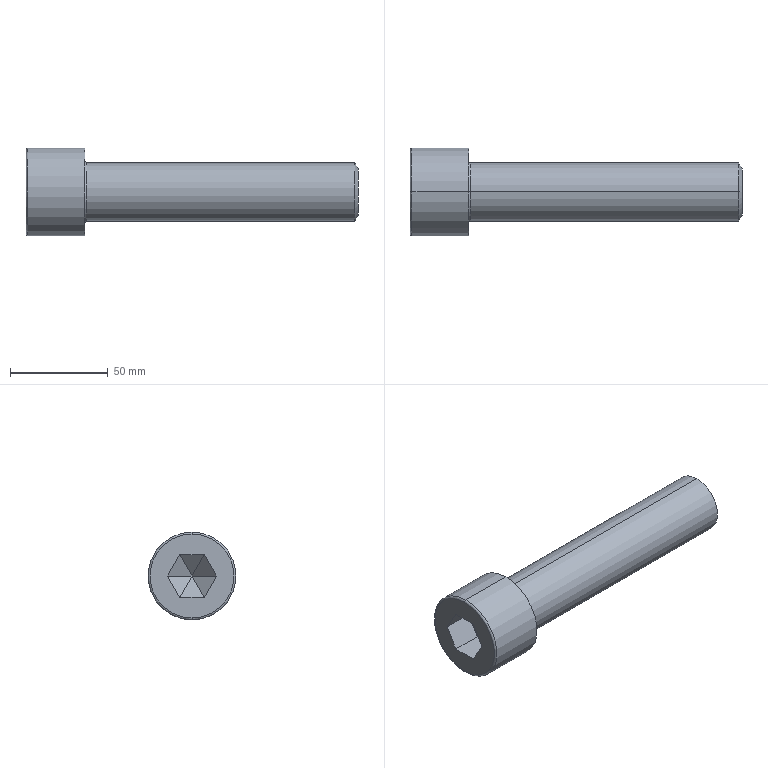Part | SolidWorks | features BlendCut 1, Cut 1, Fillet 1, LPattern 1, RevCut 1, Revolution 1 | 1 solid | 25 faces | box 170 x 45 x 45 mm | volume 138762 mm3 | plane 15 | torus 4 | cylinder 4 | cone 2 | commonest cylinder face diameters 30 x2 45 x2
STEP:
#1=CARTESIAN_POINT('',(170.,0.,11.969));
#2=VERTEX_POINT('',#1);
#3=CARTESIAN_POINT('',(170.,0.,-11.969));
#4=VERTEX_POINT('',#3);
#5=CARTESIAN_POINT('',(170.,0.,0.));
#6=DIRECTION('',(-1.,0.,0.));
#7=DIRECTION('',(0.,0.,1.));
#8=AXIS2_PLACEMENT_3D('',#5,#6,#7);
#9=CIRCLE('',#8,11.969);
#10=EDGE_CURVE('',#2,#4,#9,.T.);
#11=ORIENTED_EDGE('',*,*,#10,.T.);
#12=CARTESIAN_POINT('',(168.25,0.,-15.));
#13=VERTEX_POINT('',#12);
#14=CARTESIAN_POINT('',(168.25,0.,-15.));
#15=DIRECTION('',(-0.5,0.,-0.866));
#16=VECTOR('',#15,1000.);
#17=LINE('',#14,#16);
#18=EDGE_CURVE('',#4,#13,#17,.T.);
#19=ORIENTED_EDGE('',*,*,#18,.T.);
#20=CARTESIAN_POINT('',(168.25,0.,15.));
#21=VERTEX_POINT('',#20);
#22=CARTESIAN_POINT('',(168.25,0.,0.));
#23=DIRECTION('',(-1.,0.,0.));
#24=DIRECTION('',(0.,0.,1.));
#25=AXIS2_PLACEMENT_3D('',#22,#23,#24);
#26=CIRCLE('',#25,15.);
#27=EDGE_CURVE('',#21,#13,#26,.T.);
#28=ORIENTED_EDGE('',*,*,#27,.F.);
#29=CARTESIAN_POINT('',(168.25,0.,15.));
#30=DIRECTION('',(-0.5,0.,0.866));
#31=VECTOR('',#30,1000.);
#32=LINE('',#29,#31);
#33=EDGE_CURVE('',#2,#21,#32,.T.);
#34=ORIENTED_EDGE('',*,*,#33,.F.);
#35=EDGE_LOOP('',(#11,#19,#28,#34));
#36=FACE_OUTER_BOUND('',#35,.T.);
#37=CARTESIAN_POINT('',(168.25,0.,0.));
#38=DIRECTION('',(-1.,0.,0.));
#39=DIRECTION('',(0.,0.,1.));
#40=AXIS2_PLACEMENT_3D('',#37,#38,#39);
#41=CONICAL_SURFACE('',#40,15.,1.047);
#42=ADVANCED_FACE('',(#36),#41,.T.);
#43=CARTESIAN_POINT('',(1.,0.,-22.5));
#44=VERTEX_POINT('',#43);
#45=CARTESIAN_POINT('',(1.,0.,22.5));
#46=VERTEX_POINT('',#45);
#47=CARTESIAN_POINT('',(1.,0.,0.));
#48=DIRECTION('',(1.,0.,0.));
#49=DIRECTION('',(0.,0.,1.));
#50=AXIS2_PLACEMENT_3D('',#47,#48,#49);
#51=CIRCLE('',#50,22.5);
#52=EDGE_CURVE('',#44,#46,#51,.T.);
#53=ORIENTED_EDGE('',*,*,#52,.F.);
#54=CARTESIAN_POINT('',(0.,0.,-21.5));
#55=VERTEX_POINT('',#54);
#56=CARTESIAN_POINT('',(1.,0.,-21.5));
#57=DIRECTION('',(0.,1.,0.));
#58=DIRECTION('',(0.,0.,1.));
#59=AXIS2_PLACEMENT_3D('',#56,#57,#58);
#60=CIRCLE('',#59,1.);
#61=EDGE_CURVE('',#44,#55,#60,.T.);
#62=ORIENTED_EDGE('',*,*,#61,.T.);
#63=CARTESIAN_POINT('',(0.,0.,21.5));
#64=VERTEX_POINT('',#63);
#65=CARTESIAN_POINT('',(0.,0.,0.));
#66=DIRECTION('',(-1.,0.,0.));
#67=DIRECTION('',(0.,0.,1.));
#68=AXIS2_PLACEMENT_3D('',#65,#66,#67);
#69=CIRCLE('',#68,21.5);
#70=EDGE_CURVE('',#64,#55,#69,.T.);
#71=ORIENTED_EDGE('',*,*,#70,.F.);
#72=CARTESIAN_POINT('',(1.,0.,21.5));
#73=DIRECTION('',(0.,-1.,0.));
#74=DIRECTION('',(0.,0.,-1.));
#75=AXIS2_PLACEMENT_3D('',#72,#73,#74);
#76=CIRCLE('',#75,1.);
#77=EDGE_CURVE('',#46,#64,#76,.T.);
#78=ORIENTED_EDGE('',*,*,#77,.F.);
#79=EDGE_LOOP('',(#53,#62,#71,#78));
#80=FACE_OUTER_BOUND('',#79,.T.);
#81=CARTESIAN_POINT('',(1.,0.,0.));
#82=DIRECTION('',(-1.,0.,0.));
#83=DIRECTION('',(0.,0.,1.));
#84=AXIS2_PLACEMENT_3D('',#81,#82,#83);
#85=TOROIDAL_SURFACE('',#84,21.5,1.);
#86=ADVANCED_FACE('',(#80),#85,.T.);
#87=CARTESIAN_POINT('',(31.,0.,15.));
#88=VERTEX_POINT('',#87);
#89=CARTESIAN_POINT('',(31.,0.,-15.));
#90=VERTEX_POINT('',#89);
#91=CARTESIAN_POINT('',(31.,0.,0.));
#92=DIRECTION('',(1.,0.,0.));
#93=DIRECTION('',(0.,0.,-1.));
#94=AXIS2_PLACEMENT_3D('',#91,#92,#93);
#95=CIRCLE('',#94,15.);
#96=EDGE_CURVE('',#88,#90,#95,.T.);
#97=ORIENTED_EDGE('',*,*,#96,.F.);
#98=CARTESIAN_POINT('',(30.,0.,16.));
#99=VERTEX_POINT('',#98);
#100=CARTESIAN_POINT('',(31.,0.,16.));
#101=DIRECTION('',(0.,1.,0.));
#102=DIRECTION('',(0.,0.,1.));
#103=AXIS2_PLACEMENT_3D('',#100,#101,#102);
#104=CIRCLE('',#103,1.);
#105=EDGE_CURVE('',#88,#99,#104,.T.);
#106=ORIENTED_EDGE('',*,*,#105,.T.);
#107=CARTESIAN_POINT('',(30.,0.,-16.));
#108=VERTEX_POINT('',#107);
#109=CARTESIAN_POINT('',(30.,0.,0.));
#110=DIRECTION('',(1.,0.,0.));
#111=DIRECTION('',(0.,0.,-1.));
#112=AXIS2_PLACEMENT_3D('',#109,#110,#111);
#113=CIRCLE('',#112,16.);
#114=EDGE_CURVE('',#99,#108,#113,.T.);
#115=ORIENTED_EDGE('',*,*,#114,.T.);
#116=CARTESIAN_POINT('',(31.,0.,-16.));
#117=DIRECTION('',(0.,-1.,0.));
#118=DIRECTION('',(0.,0.,-1.));
#119=AXIS2_PLACEMENT_3D('',#116,#117,#118);
#120=CIRCLE('',#119,1.);
#121=EDGE_CURVE('',#90,#108,#120,.T.);
#122=ORIENTED_EDGE('',*,*,#121,.F.);
#123=EDGE_LOOP('',(#97,#106,#115,#122));
#124=FACE_OUTER_BOUND('',#123,.T.);
#125=CARTESIAN_POINT('',(31.,0.,0.));
#126=DIRECTION('',(1.,0.,0.));
#127=DIRECTION('',(0.,0.,-1.));
#128=AXIS2_PLACEMENT_3D('',#125,#126,#127);
#129=TOROIDAL_SURFACE('',#128,16.,1.);
#130=ADVANCED_FACE('',(#124),#129,.F.);
#131=ORIENTED_EDGE('',*,*,#52,.T.);
#132=CARTESIAN_POINT('',(30.,0.,22.5));
#133=VERTEX_POINT('',#132);
#134=CARTESIAN_POINT('',(0.,0.,22.5));
#135=DIRECTION('',(1.,0.,0.));
#136=VECTOR('',#135,1000.);
#137=LINE('',#134,#136);
#138=EDGE_CURVE('',#46,#133,#137,.T.);
#139=ORIENTED_EDGE('',*,*,#138,.T.);
#140=CARTESIAN_POINT('',(30.,0.,-22.5));
#141=VERTEX_POINT('',#140);
#142=CARTESIAN_POINT('',(30.,0.,0.));
#143=DIRECTION('',(1.,0.,0.));
#144=DIRECTION('',(0.,0.,-1.));
#145=AXIS2_PLACEMENT_3D('',#142,#143,#144);
#146=CIRCLE('',#145,22.5);
#147=EDGE_CURVE('',#141,#133,#146,.T.);
#148=ORIENTED_EDGE('',*,*,#147,.F.);
#149=CARTESIAN_POINT('',(0.,0.,-22.5));
#150=DIRECTION('',(1.,0.,0.));
#151=VECTOR('',#150,1000.);
#152=LINE('',#149,#151);
#153=EDGE_CURVE('',#44,#141,#152,.T.);
#154=ORIENTED_EDGE('',*,*,#153,.F.);
#155=EDGE_LOOP('',(#131,#139,#148,#154));
#156=FACE_OUTER_BOUND('',#155,.T.);
#157=CARTESIAN_POINT('',(0.,0.,0.));
#158=DIRECTION('',(1.,0.,0.));
#159=DIRECTION('',(0.,0.,-1.));
#160=AXIS2_PLACEMENT_3D('',#157,#158,#159);
#161=CYLINDRICAL_SURFACE('',#160,22.5);
#162=ADVANCED_FACE('',(#156),#161,.T.);
#163=CARTESIAN_POINT('',(31.,0.,0.));
#164=DIRECTION('',(1.,0.,0.));
#165=DIRECTION('',(0.,0.,-1.));
#166=AXIS2_PLACEMENT_3D('',#163,#164,#165);
#167=CIRCLE('',#166,15.);
#168=EDGE_CURVE('',#90,#88,#167,.T.);
#169=ORIENTED_EDGE('',*,*,#168,.T.);
#170=CARTESIAN_POINT('',(0.,0.,15.));
#171=DIRECTION('',(1.,0.,0.));
#172=VECTOR('',#171,1000.);
#173=LINE('',#170,#172);
#174=EDGE_CURVE('',#88,#21,#173,.T.);
#175=ORIENTED_EDGE('',*,*,#174,.T.);
#176=ORIENTED_EDGE('',*,*,#27,.T.);
#177=CARTESIAN_POINT('',(0.,0.,-15.));
#178=DIRECTION('',(1.,0.,0.));
#179=VECTOR('',#178,1000.);
#180=LINE('',#177,#179);
#181=EDGE_CURVE('',#90,#13,#180,.T.);
#182=ORIENTED_EDGE('',*,*,#181,.F.);
#183=EDGE_LOOP('',(#169,#175,#176,#182));
#184=FACE_OUTER_BOUND('',#183,.T.);
#185=CARTESIAN_POINT('',(0.,0.,0.));
#186=DIRECTION('',(1.,0.,0.));
#187=DIRECTION('',(0.,0.,-1.));
#188=AXIS2_PLACEMENT_3D('',#185,#186,#187);
#189=CYLINDRICAL_SURFACE('',#188,15.);
#190=ADVANCED_FACE('',(#184),#189,.T.);
#191=ORIENTED_EDGE('',*,*,#174,.F.);
#192=ORIENTED_EDGE('',*,*,#96,.T.);
#193=ORIENTED_EDGE('',*,*,#181,.T.);
#194=CARTESIAN_POINT('',(168.25,0.,0.));
#195=DIRECTION('',(-1.,0.,0.));
#196=DIRECTION('',(0.,0.,1.));
#197=AXIS2_PLACEMENT_3D('',#194,#195,#196);
#198=CIRCLE('',#197,15.);
#199=EDGE_CURVE('',#13,#21,#198,.T.);
#200=ORIENTED_EDGE('',*,*,#199,.T.);
#201=EDGE_LOOP('',(#191,#192,#193,#200));
#202=FACE_OUTER_BOUND('',#201,.T.);
#203=CARTESIAN_POINT('',(0.,0.,0.));
#204=DIRECTION('',(1.,0.,0.));
#205=DIRECTION('',(0.,0.,-1.));
#206=AXIS2_PLACEMENT_3D('',#203,#204,#205);
#207=CYLINDRICAL_SURFACE('',#206,15.);
#208=ADVANCED_FACE('',(#202),#207,.T.);
#209=ORIENTED_EDGE('',*,*,#70,.T.);
#210=CARTESIAN_POINT('',(0.,0.,0.));
#211=DIRECTION('',(-1.,0.,0.));
#212=DIRECTION('',(0.,0.,1.));
#213=AXIS2_PLACEMENT_3D('',#210,#211,#212);
#214=CIRCLE('',#213,21.5);
#215=EDGE_CURVE('',#55,#64,#214,.T.);
#216=ORIENTED_EDGE('',*,*,#215,.T.);
#217=EDGE_LOOP('',(#209,#216));
#218=FACE_OUTER_BOUND('',#217,.T.);
#219=CARTESIAN_POINT('',(0.,-12.575,0.));
#220=VERTEX_POINT('',#219);
#221=CARTESIAN_POINT('',(0.,-6.288,10.89));
#222=VERTEX_POINT('',#221);
#223=CARTESIAN_POINT('',(0.,-12.575,0.));
#224=DIRECTION('',(0.,0.5,0.866));
#225=VECTOR('',#224,1000.);
#226=LINE('',#223,#225);
#227=EDGE_CURVE('',#220,#222,#226,.T.);
#228=ORIENTED_EDGE('',*,*,#227,.F.);
#229=CARTESIAN_POINT('',(0.,-6.287,-10.89));
#230=VERTEX_POINT('',#229);
#231=CARTESIAN_POINT('',(0.,-6.287,-10.89));
#232=DIRECTION('',(0.,-0.5,0.866));
#233=VECTOR('',#232,1000.);
#234=LINE('',#231,#233);
#235=EDGE_CURVE('',#230,#220,#234,.T.);
#236=ORIENTED_EDGE('',*,*,#235,.F.);
#237=CARTESIAN_POINT('',(0.,6.288,-10.89));
#238=VERTEX_POINT('',#237);
#239=CARTESIAN_POINT('',(0.,6.288,-10.89));
#240=DIRECTION('',(0.,-1.,0.));
#241=VECTOR('',#240,1000.);
#242=LINE('',#239,#241);
#243=EDGE_CURVE('',#238,#230,#242,.T.);
#244=ORIENTED_EDGE('',*,*,#243,.F.);
#245=CARTESIAN_POINT('',(0.,12.575,0.));
#246=VERTEX_POINT('',#245);
#247=CARTESIAN_POINT('',(0.,12.575,0.));
#248=DIRECTION('',(0.,-0.5,-0.866));
#249=VECTOR('',#248,1000.);
#250=LINE('',#247,#249);
#251=EDGE_CURVE('',#246,#238,#250,.T.);
#252=ORIENTED_EDGE('',*,*,#251,.F.);
#253=CARTESIAN_POINT('',(0.,6.288,10.89));
#254=VERTEX_POINT('',#253);
#255=CARTESIAN_POINT('',(0.,6.288,10.89));
#256=DIRECTION('',(0.,0.5,-0.866));
#257=VECTOR('',#256,1000.);
#258=LINE('',#255,#257);
#259=EDGE_CURVE('',#254,#246,#258,.T.);
#260=ORIENTED_EDGE('',*,*,#259,.F.);
#261=CARTESIAN_POINT('',(0.,-6.288,10.89));
#262=DIRECTION('',(0.,1.,0.));
#263=VECTOR('',#262,1000.);
#264=LINE('',#261,#263);
#265=EDGE_CURVE('',#222,#254,#264,.T.);
#266=ORIENTED_EDGE('',*,*,#265,.F.);
#267=EDGE_LOOP('',(#228,#236,#244,#252,#260,#266));
#268=FACE_BOUND('',#267,.T.);
#269=CARTESIAN_POINT('',(0.,0.,0.));
#270=DIRECTION('',(-1.,0.,0.));
#271=DIRECTION('',(0.,0.,1.));
#272=AXIS2_PLACEMENT_3D('',#269,#270,#271);
#273=PLANE('',#272);
#274=ADVANCED_FACE('',(#218,#268),#273,.T.);
#275=ORIENTED_EDGE('',*,*,#138,.F.);
#276=CARTESIAN_POINT('',(1.,0.,0.));
#277=DIRECTION('',(1.,0.,0.));
#278=DIRECTION('',(0.,0.,1.));
#279=AXIS2_PLACEMENT_3D('',#276,#277,#278);
#280=CIRCLE('',#279,22.5);
#281=EDGE_CURVE('',#46,#44,#280,.T.);
#282=ORIENTED_EDGE('',*,*,#281,.T.);
#283=ORIENTED_EDGE('',*,*,#153,.T.);
#284=CARTESIAN_POINT('',(30.,0.,0.));
#285=DIRECTION('',(1.,0.,0.));
#286=DIRECTION('',(0.,0.,-1.));
#287=AXIS2_PLACEMENT_3D('',#284,#285,#286);
#288=CIRCLE('',#287,22.5);
#289=EDGE_CURVE('',#133,#141,#288,.T.);
#290=ORIENTED_EDGE('',*,*,#289,.F.);
#291=EDGE_LOOP('',(#275,#282,#283,#290));
#292=FACE_OUTER_BOUND('',#291,.T.);
#293=CARTESIAN_POINT('',(0.,0.,0.));
#294=DIRECTION('',(1.,0.,0.));
#295=DIRECTION('',(0.,0.,-1.));
#296=AXIS2_PLACEMENT_3D('',#293,#294,#295);
#297=CYLINDRICAL_SURFACE('',#296,22.5);
#298=ADVANCED_FACE('',(#292),#297,.T.);
#299=ORIENTED_EDGE('',*,*,#147,.T.);
#300=ORIENTED_EDGE('',*,*,#289,.T.);
#301=EDGE_LOOP('',(#299,#300));
#302=FACE_OUTER_BOUND('',#301,.T.);
#303=CARTESIAN_POINT('',(30.,0.,0.));
#304=DIRECTION('',(1.,0.,0.));
#305=DIRECTION('',(0.,0.,-1.));
#306=AXIS2_PLACEMENT_3D('',#303,#304,#305);
#307=CIRCLE('',#306,16.);
#308=EDGE_CURVE('',#108,#99,#307,.T.);
#309=ORIENTED_EDGE('',*,*,#308,.F.);
#310=ORIENTED_EDGE('',*,*,#114,.F.);
#311=EDGE_LOOP('',(#309,#310));
#312=FACE_BOUND('',#311,.T.);
#313=CARTESIAN_POINT('',(30.,22.5,0.));
#314=DIRECTION('',(1.,0.,0.));
#315=DIRECTION('',(0.,0.,-1.));
#316=AXIS2_PLACEMENT_3D('',#313,#314,#315);
#317=PLANE('',#316);
#318=ADVANCED_FACE('',(#302,#312),#317,.T.);
#319=ORIENTED_EDGE('',*,*,#105,.F.);
#320=ORIENTED_EDGE('',*,*,#168,.F.);
#321=ORIENTED_EDGE('',*,*,#121,.T.);
#322=ORIENTED_EDGE('',*,*,#308,.T.);
#323=EDGE_LOOP('',(#319,#320,#321,#322));
#324=FACE_OUTER_BOUND('',#323,.T.);
#325=CARTESIAN_POINT('',(31.,0.,0.));
#326=DIRECTION('',(1.,0.,0.));
#327=DIRECTION('',(0.,0.,-1.));
#328=AXIS2_PLACEMENT_3D('',#325,#326,#327);
#329=TOROIDAL_SURFACE('',#328,16.,1.);
#330=ADVANCED_FACE('',(#324),#329,.F.);
#331=ORIENTED_EDGE('',*,*,#227,.T.);
#332=CARTESIAN_POINT('',(15.5,-6.288,10.89));
#333=VERTEX_POINT('',#332);
#334=CARTESIAN_POINT('',(15.5,-6.288,10.89));
#335=DIRECTION('',(-1.,0.,0.));
#336=VECTOR('',#335,1000.);
#337=LINE('',#334,#336);
#338=EDGE_CURVE('',#333,#222,#337,.T.);
#339=ORIENTED_EDGE('',*,*,#338,.F.);
#340=CARTESIAN_POINT('',(15.5,-12.575,0.));
#341=VERTEX_POINT('',#340);
#342=CARTESIAN_POINT('',(15.5,-12.575,0.));
#343=DIRECTION('',(0.,0.5,0.866));
#344=VECTOR('',#343,1000.);
#345=LINE('',#342,#344);
#346=EDGE_CURVE('',#341,#333,#345,.T.);
#347=ORIENTED_EDGE('',*,*,#346,.F.);
#348=CARTESIAN_POINT('',(15.5,-12.575,0.));
#349=DIRECTION('',(-1.,0.,0.));
#350=VECTOR('',#349,1000.);
#351=LINE('',#348,#350);
#352=EDGE_CURVE('',#341,#220,#351,.T.);
#353=ORIENTED_EDGE('',*,*,#352,.T.);
#354=EDGE_LOOP('',(#331,#339,#347,#353));
#355=FACE_OUTER_BOUND('',#354,.T.);
#356=CARTESIAN_POINT('',(15.5,-12.575,0.));
#357=DIRECTION('',(0.,-0.866,0.5));
#358=DIRECTION('',(0.,-0.5,-0.866));
#359=AXIS2_PLACEMENT_3D('',#356,#357,#358);
#360=PLANE('',#359);
#361=ADVANCED_FACE('',(#355),#360,.F.);
#362=ORIENTED_EDGE('',*,*,#235,.T.);
#363=ORIENTED_EDGE('',*,*,#352,.F.);
#364=CARTESIAN_POINT('',(15.5,-6.287,-10.89));
#365=VERTEX_POINT('',#364);
#366=CARTESIAN_POINT('',(15.5,-6.287,-10.89));
#367=DIRECTION('',(0.,-0.5,0.866));
#368=VECTOR('',#367,1000.);
#369=LINE('',#366,#368);
#370=EDGE_CURVE('',#365,#341,#369,.T.);
#371=ORIENTED_EDGE('',*,*,#370,.F.);
#372=CARTESIAN_POINT('',(15.5,-6.287,-10.89));
#373=DIRECTION('',(-1.,0.,0.));
#374=VECTOR('',#373,1000.);
#375=LINE('',#372,#374);
#376=EDGE_CURVE('',#365,#230,#375,.T.);
#377=ORIENTED_EDGE('',*,*,#376,.T.);
#378=EDGE_LOOP('',(#362,#363,#371,#377));
#379=FACE_OUTER_BOUND('',#378,.T.);
#380=CARTESIAN_POINT('',(15.5,-6.287,-10.89));
#381=DIRECTION('',(0.,-0.866,-0.5));
#382=DIRECTION('',(0.,0.5,-0.866));
#383=AXIS2_PLACEMENT_3D('',#380,#381,#382);
#384=PLANE('',#383);
#385=ADVANCED_FACE('',(#379),#384,.F.);
#386=ORIENTED_EDGE('',*,*,#243,.T.);
#387=ORIENTED_EDGE('',*,*,#376,.F.);
#388=CARTESIAN_POINT('',(15.5,6.288,-10.89));
#389=VERTEX_POINT('',#388);
#390=CARTESIAN_POINT('',(15.5,6.288,-10.89));
#391=DIRECTION('',(0.,-1.,0.));
#392=VECTOR('',#391,1000.);
#393=LINE('',#390,#392);
#394=EDGE_CURVE('',#389,#365,#393,.T.);
#395=ORIENTED_EDGE('',*,*,#394,.F.);
#396=CARTESIAN_POINT('',(15.5,6.288,-10.89));
#397=DIRECTION('',(-1.,0.,0.));
#398=VECTOR('',#397,1000.);
#399=LINE('',#396,#398);
#400=EDGE_CURVE('',#389,#238,#399,.T.);
#401=ORIENTED_EDGE('',*,*,#400,.T.);
#402=EDGE_LOOP('',(#386,#387,#395,#401));
#403=FACE_OUTER_BOUND('',#402,.T.);
#404=CARTESIAN_POINT('',(15.5,6.288,-10.89));
#405=DIRECTION('',(0.,0.,-1.));
#406=DIRECTION('',(0.,1.,0.));
#407=AXIS2_PLACEMENT_3D('',#404,#405,#406);
#408=PLANE('',#407);
#409=ADVANCED_FACE('',(#403),#408,.F.);
#410=ORIENTED_EDGE('',*,*,#251,.T.);
#411=ORIENTED_EDGE('',*,*,#400,.F.);
#412=CARTESIAN_POINT('',(15.5,12.575,0.));
#413=VERTEX_POINT('',#412);
#414=CARTESIAN_POINT('',(15.5,12.575,0.));
#415=DIRECTION('',(0.,-0.5,-0.866));
#416=VECTOR('',#415,1000.);
#417=LINE('',#414,#416);
#418=EDGE_CURVE('',#413,#389,#417,.T.);
#419=ORIENTED_EDGE('',*,*,#418,.F.);
#420=CARTESIAN_POINT('',(15.5,12.575,0.));
#421=DIRECTION('',(-1.,0.,0.));
#422=VECTOR('',#421,1000.);
#423=LINE('',#420,#422);
#424=EDGE_CURVE('',#413,#246,#423,.T.);
#425=ORIENTED_EDGE('',*,*,#424,.T.);
#426=EDGE_LOOP('',(#410,#411,#419,#425));
#427=FACE_OUTER_BOUND('',#426,.T.);
#428=CARTESIAN_POINT('',(15.5,12.575,0.));
#429=DIRECTION('',(0.,0.866,-0.5));
#430=DIRECTION('',(0.,0.5,0.866));
#431=AXIS2_PLACEMENT_3D('',#428,#429,#430);
#432=PLANE('',#431);
#433=ADVANCED_FACE('',(#427),#432,.F.);
#434=ORIENTED_EDGE('',*,*,#259,.T.);
#435=ORIENTED_EDGE('',*,*,#424,.F.);
#436=CARTESIAN_POINT('',(15.5,6.287,10.89));
#437=VERTEX_POINT('',#436);
#438=CARTESIAN_POINT('',(15.5,6.288,10.89));
#439=DIRECTION('',(0.,0.5,-0.866));
#440=VECTOR('',#439,1000.);
#441=LINE('',#438,#440);
#442=EDGE_CURVE('',#437,#413,#441,.T.);
#443=ORIENTED_EDGE('',*,*,#442,.F.);
#444=CARTESIAN_POINT('',(15.5,6.288,10.89));
#445=DIRECTION('',(-1.,0.,0.));
#446=VECTOR('',#445,1000.);
#447=LINE('',#444,#446);
#448=EDGE_CURVE('',#437,#254,#447,.T.);
#449=ORIENTED_EDGE('',*,*,#448,.T.);
#450=EDGE_LOOP('',(#434,#435,#443,#449));
#451=FACE_OUTER_BOUND('',#450,.T.);
#452=CARTESIAN_POINT('',(15.5,6.288,10.89));
#453=DIRECTION('',(0.,0.866,0.5));
#454=DIRECTION('',(0.,-0.5,0.866));
#455=AXIS2_PLACEMENT_3D('',#452,#453,#454);
#456=PLANE('',#455);
#457=ADVANCED_FACE('',(#451),#456,.F.);
#458=ORIENTED_EDGE('',*,*,#265,.T.);
#459=ORIENTED_EDGE('',*,*,#448,.F.);
#460=CARTESIAN_POINT('',(15.5,-6.288,10.89));
#461=DIRECTION('',(0.,1.,0.));
#462=VECTOR('',#461,1000.);
#463=LINE('',#460,#462);
#464=EDGE_CURVE('',#333,#437,#463,.T.);
#465=ORIENTED_EDGE('',*,*,#464,.F.);
#466=ORIENTED_EDGE('',*,*,#338,.T.);
#467=EDGE_LOOP('',(#458,#459,#465,#466));
#468=FACE_OUTER_BOUND('',#467,.T.);
#469=CARTESIAN_POINT('',(15.5,-6.288,10.89));
#470=DIRECTION('',(0.,0.,1.));
#471=DIRECTION('',(0.,-1.,0.));
#472=AXIS2_PLACEMENT_3D('',#469,#470,#471);
#473=PLANE('',#472);
#474=ADVANCED_FACE('',(#468),#473,.F.);
#475=CARTESIAN_POINT('',(25.,0.,0.));
#476=VERTEX_POINT('',#475);
#477=CARTESIAN_POINT('',(25.,0.,0.));
#478=DIRECTION('',(-0.6028,-0.7979,0.));
#479=VECTOR('',#478,1000.);
#480=LINE('',#477,#479);
#481=EDGE_CURVE('',#476,#341,#480,.T.);
#482=ORIENTED_EDGE('',*,*,#481,.F.);
#483=CARTESIAN_POINT('',(25.,0.,0.));
#484=DIRECTION('',(-0.6028,-0.399,-0.691));
#485=VECTOR('',#484,1000.);
#486=LINE('',#483,#485);
#487=EDGE_CURVE('',#476,#365,#486,.T.);
#488=ORIENTED_EDGE('',*,*,#487,.T.);
#489=ORIENTED_EDGE('',*,*,#370,.T.);
#490=EDGE_LOOP('',(#482,#488,#489));
#491=FACE_OUTER_BOUND('',#490,.T.);
#492=CARTESIAN_POINT('',(15.5,-12.575,0.));
#493=DIRECTION('',(-0.7536,0.5693,0.3287));
#494=DIRECTION('',(-0.6028,-0.7979,0.));
#495=AXIS2_PLACEMENT_3D('',#492,#493,#494);
#496=PLANE('',#495);
#497=ADVANCED_FACE('',(#491),#496,.T.);
#498=ORIENTED_EDGE('',*,*,#487,.F.);
#499=CARTESIAN_POINT('',(25.,0.,0.));
#500=DIRECTION('',(-0.6028,0.399,-0.691));
#501=VECTOR('',#500,1000.);
#502=LINE('',#499,#501);
#503=EDGE_CURVE('',#476,#389,#502,.T.);
#504=ORIENTED_EDGE('',*,*,#503,.T.);
#505=ORIENTED_EDGE('',*,*,#394,.T.);
#506=EDGE_LOOP('',(#498,#504,#505));
#507=FACE_OUTER_BOUND('',#506,.T.);
#508=CARTESIAN_POINT('',(15.5,-6.287,-10.89));
#509=DIRECTION('',(-0.7536,0.,0.6574));
#510=DIRECTION('',(0.6574,0.,0.7536));
#511=AXIS2_PLACEMENT_3D('',#508,#509,#510);
#512=PLANE('',#511);
#513=ADVANCED_FACE('',(#507),#512,.T.);
#514=CARTESIAN_POINT('',(25.,0.,0.));
#515=DIRECTION('',(-0.6028,-0.399,0.691));
#516=VECTOR('',#515,1000.);
#517=LINE('',#514,#516);
#518=EDGE_CURVE('',#476,#333,#517,.T.);
#519=ORIENTED_EDGE('',*,*,#518,.F.);
#520=ORIENTED_EDGE('',*,*,#481,.T.);
#521=ORIENTED_EDGE('',*,*,#346,.T.);
#522=EDGE_LOOP('',(#519,#520,#521));
#523=FACE_OUTER_BOUND('',#522,.T.);
#524=CARTESIAN_POINT('',(15.5,-6.288,10.89));
#525=DIRECTION('',(-0.7536,0.5693,-0.3287));
#526=DIRECTION('',(-0.6028,-0.7979,0.));
#527=AXIS2_PLACEMENT_3D('',#524,#525,#526);
#528=PLANE('',#527);
#529=ADVANCED_FACE('',(#523),#528,.T.);
#530=ORIENTED_EDGE('',*,*,#503,.F.);
#531=CARTESIAN_POINT('',(25.,0.,0.));
#532=DIRECTION('',(-0.6028,0.7979,0.));
#533=VECTOR('',#532,1000.);
#534=LINE('',#531,#533);
#535=EDGE_CURVE('',#476,#413,#534,.T.);
#536=ORIENTED_EDGE('',*,*,#535,.T.);
#537=ORIENTED_EDGE('',*,*,#418,.T.);
#538=EDGE_LOOP('',(#530,#536,#537));
#539=FACE_OUTER_BOUND('',#538,.T.);
#540=CARTESIAN_POINT('',(15.5,6.288,-10.89));
#541=DIRECTION('',(-0.7536,-0.5693,0.3287));
#542=DIRECTION('',(0.6028,-0.7979,0.));
#543=AXIS2_PLACEMENT_3D('',#540,#541,#542);
#544=PLANE('',#543);
#545=ADVANCED_FACE('',(#539),#544,.T.);
#546=CARTESIAN_POINT('',(25.,0.,0.));
#547=DIRECTION('',(-0.6028,0.399,0.691));
#548=VECTOR('',#547,1000.);
#549=LINE('',#546,#548);
#550=EDGE_CURVE('',#476,#437,#549,.T.);
#551=ORIENTED_EDGE('',*,*,#550,.F.);
#552=ORIENTED_EDGE('',*,*,#518,.T.);
#553=ORIENTED_EDGE('',*,*,#464,.T.);
#554=EDGE_LOOP('',(#551,#552,#553));
#555=FACE_OUTER_BOUND('',#554,.T.);
#556=CARTESIAN_POINT('',(15.5,6.288,10.89));
#557=DIRECTION('',(-0.7536,0.,-0.6574));
#558=DIRECTION('',(-0.6574,0.,0.7536));
#559=AXIS2_PLACEMENT_3D('',#556,#557,#558);
#560=PLANE('',#559);
#561=ADVANCED_FACE('',(#555),#560,.T.);
#562=ORIENTED_EDGE('',*,*,#535,.F.);
#563=ORIENTED_EDGE('',*,*,#550,.T.);
#564=ORIENTED_EDGE('',*,*,#442,.T.);
#565=EDGE_LOOP('',(#562,#563,#564));
#566=FACE_OUTER_BOUND('',#565,.T.);
#567=CARTESIAN_POINT('',(15.5,12.575,0.));
#568=DIRECTION('',(-0.7536,-0.5693,-0.3287));
#569=DIRECTION('',(0.6028,-0.7979,0.));
#570=AXIS2_PLACEMENT_3D('',#567,#568,#569);
#571=PLANE('',#570);
#572=ADVANCED_FACE('',(#566),#571,.T.);
#573=ORIENTED_EDGE('',*,*,#61,.F.);
#574=ORIENTED_EDGE('',*,*,#281,.F.);
#575=ORIENTED_EDGE('',*,*,#77,.T.);
#576=ORIENTED_EDGE('',*,*,#215,.F.);
#577=EDGE_LOOP('',(#573,#574,#575,#576));
#578=FACE_OUTER_BOUND('',#577,.T.);
#579=CARTESIAN_POINT('',(1.,0.,0.));
#580=DIRECTION('',(-1.,0.,0.));
#581=DIRECTION('',(0.,0.,1.));
#582=AXIS2_PLACEMENT_3D('',#579,#580,#581);
#583=TOROIDAL_SURFACE('',#582,21.5,1.);
#584=ADVANCED_FACE('',(#578),#583,.T.);
#585=ORIENTED_EDGE('',*,*,#18,.F.);
#586=CARTESIAN_POINT('',(170.,0.,0.));
#587=DIRECTION('',(-1.,0.,0.));
#588=DIRECTION('',(0.,0.,1.));
#589=AXIS2_PLACEMENT_3D('',#586,#587,#588);
#590=CIRCLE('',#589,11.969);
#591=EDGE_CURVE('',#4,#2,#590,.T.);
#592=ORIENTED_EDGE('',*,*,#591,.T.);
#593=ORIENTED_EDGE('',*,*,#33,.T.);
#594=ORIENTED_EDGE('',*,*,#199,.F.);
#595=EDGE_LOOP('',(#585,#592,#593,#594));
#596=FACE_OUTER_BOUND('',#595,.T.);
#597=CARTESIAN_POINT('',(168.25,0.,0.));
#598=DIRECTION('',(-1.,0.,0.));
#599=DIRECTION('',(0.,0.,1.));
#600=AXIS2_PLACEMENT_3D('',#597,#598,#599);
#601=CONICAL_SURFACE('',#600,15.,1.047);
#602=ADVANCED_FACE('',(#596),#601,.T.);
#603=ORIENTED_EDGE('',*,*,#10,.F.);
#604=ORIENTED_EDGE('',*,*,#591,.F.);
#605=EDGE_LOOP('',(#603,#604));
#606=FACE_OUTER_BOUND('',#605,.T.);
#607=CARTESIAN_POINT('',(170.,15.,0.));
#608=DIRECTION('',(1.,0.,0.));
#609=DIRECTION('',(0.,0.,-1.));
#610=AXIS2_PLACEMENT_3D('',#607,#608,#609);
#611=PLANE('',#610);
#612=ADVANCED_FACE('',(#606),#611,.T.);
#613=CLOSED_SHELL('',(#42,#86,#130,#162,#190,#208,#274,#298,#318,#330,#361,#385,#409,#433,#457,#474,#497,#513,#529,#545,#561,#572,#584,#602,#612));
#614=MANIFOLD_SOLID_BREP('',#613);
#615=CARTESIAN_POINT('',(0.,0.,0.));
#616=DIRECTION('',(0.,0.,1.));
#617=DIRECTION('',(1.,0.,0.));
#618=AXIS2_PLACEMENT_3D('',#615,#616,#617);
#619=(LENGTH_UNIT()NAMED_UNIT(*)SI_UNIT(.MILLI.,.METRE.));
#620=UNCERTAINTY_MEASURE_WITH_UNIT(LENGTH_MEASURE(0.00001),#619,'','');
#621=(NAMED_UNIT(*)PLANE_ANGLE_UNIT()SI_UNIT($,.RADIAN.));
#622=(NAMED_UNIT(*)SI_UNIT($,.STERADIAN.)SOLID_ANGLE_UNIT());
#623=(GEOMETRIC_REPRESENTATION_CONTEXT(3)GLOBAL_UNCERTAINTY_ASSIGNED_CONTEXT((#620))GLOBAL_UNIT_ASSIGNED_CONTEXT((#619,#621,#622))REPRESENTATION_CONTEXT('',''));
#624=ADVANCED_BREP_SHAPE_REPRESENTATION('',(#614,#618),#623);